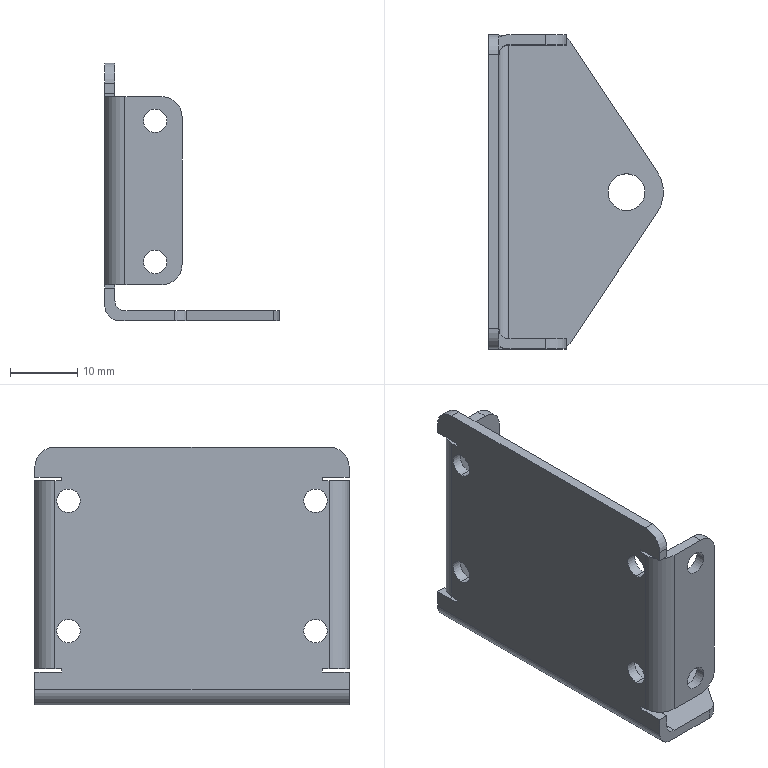Part | STEP file | ABA 47-1 - Lateral | 1 solid | 62 faces | box 26 x 46.8 x 38.4 mm | volume 4492 mm3 | cylinder 33 | plane 29 | commonest cylinder face diameters 3.5 x16 6 x8 3 x3 4 x2 5.5 x2 4.5 x1